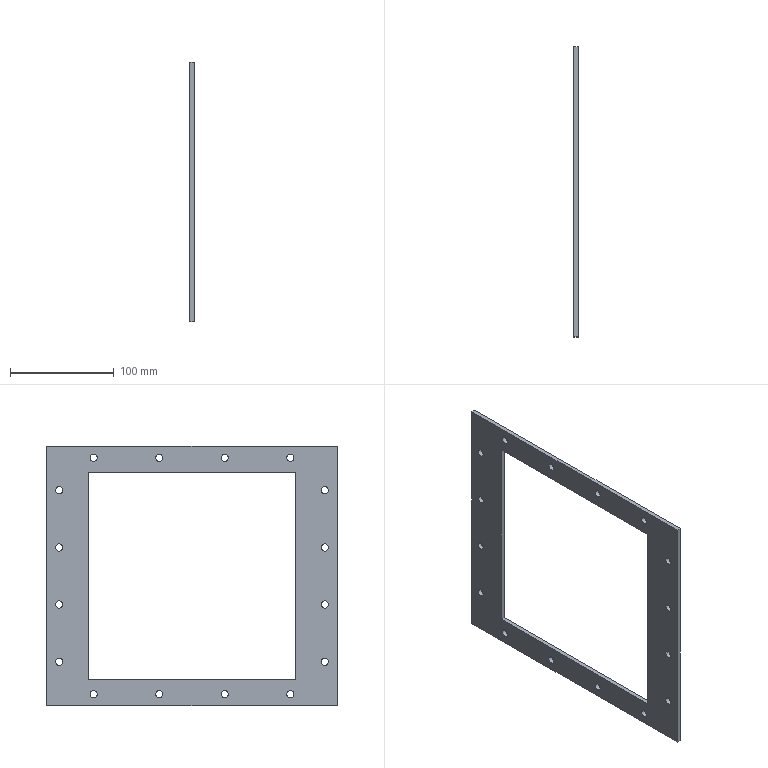Part | SolidWorks | features Boss 6, ICE 3, Revolution 3, CirPattern 2, Cut 2, Extrusion 1, MirrorPattern 1, RevCut 1, Shell 1 | 1 solid | 42 faces | box 4 x 280 x 250 mm | volume 117537 mm3 | cylinder 32 | plane 10 | commonest cylinder face diameters 7 x32
STEP:
#1=CARTESIAN_POINT('',(-187.,-320.5,-82.533));
#2=VERTEX_POINT('',#1);
#3=CARTESIAN_POINT('',(-187.,-327.5,-82.533));
#4=VERTEX_POINT('',#3);
#5=CARTESIAN_POINT('',(-187.,-324.,-82.533));
#6=DIRECTION('',(-1.,0.,0.));
#7=DIRECTION('',(0.,-1.,0.));
#8=AXIS2_PLACEMENT_3D('',#5,#6,#7);
#9=CIRCLE('',#8,3.5);
#10=EDGE_CURVE('',#2,#4,#9,.T.);
#11=ORIENTED_EDGE('',*,*,#10,.F.);
#12=CARTESIAN_POINT('',(-191.,-320.5,-82.533));
#13=VERTEX_POINT('',#12);
#14=CARTESIAN_POINT('',(-181.,-320.5,-82.533));
#15=DIRECTION('',(-1.,0.,0.));
#16=VECTOR('',#15,1000.);
#17=LINE('',#14,#16);
#18=EDGE_CURVE('',#2,#13,#17,.T.);
#19=ORIENTED_EDGE('',*,*,#18,.T.);
#20=CARTESIAN_POINT('',(-191.,-327.5,-82.533));
#21=VERTEX_POINT('',#20);
#22=CARTESIAN_POINT('',(-191.,-324.,-82.533));
#23=DIRECTION('',(-1.,0.,0.));
#24=DIRECTION('',(0.,1.,0.));
#25=AXIS2_PLACEMENT_3D('',#22,#23,#24);
#26=CIRCLE('',#25,3.5);
#27=EDGE_CURVE('',#13,#21,#26,.T.);
#28=ORIENTED_EDGE('',*,*,#27,.T.);
#29=CARTESIAN_POINT('',(-181.,-327.5,-82.533));
#30=DIRECTION('',(-1.,0.,0.));
#31=VECTOR('',#30,1000.);
#32=LINE('',#29,#31);
#33=EDGE_CURVE('',#4,#21,#32,.T.);
#34=ORIENTED_EDGE('',*,*,#33,.F.);
#35=EDGE_LOOP('',(#11,#19,#28,#34));
#36=FACE_OUTER_BOUND('',#35,.T.);
#37=CARTESIAN_POINT('',(-181.,-324.,-82.533));
#38=DIRECTION('',(-1.,0.,0.));
#39=DIRECTION('',(0.,-1.,0.));
#40=AXIS2_PLACEMENT_3D('',#37,#38,#39);
#41=CYLINDRICAL_SURFACE('',#40,3.5);
#42=ADVANCED_FACE('',(#36),#41,.F.);
#43=CARTESIAN_POINT('',(-187.,-320.5,-27.511));
#44=VERTEX_POINT('',#43);
#45=CARTESIAN_POINT('',(-187.,-327.5,-27.511));
#46=VERTEX_POINT('',#45);
#47=CARTESIAN_POINT('',(-187.,-324.,-27.511));
#48=DIRECTION('',(-1.,0.,0.));
#49=DIRECTION('',(0.,-1.,0.));
#50=AXIS2_PLACEMENT_3D('',#47,#48,#49);
#51=CIRCLE('',#50,3.5);
#52=EDGE_CURVE('',#44,#46,#51,.T.);
#53=ORIENTED_EDGE('',*,*,#52,.F.);
#54=CARTESIAN_POINT('',(-191.,-320.5,-27.511));
#55=VERTEX_POINT('',#54);
#56=CARTESIAN_POINT('',(-181.,-320.5,-27.511));
#57=DIRECTION('',(-1.,0.,0.));
#58=VECTOR('',#57,1000.);
#59=LINE('',#56,#58);
#60=EDGE_CURVE('',#44,#55,#59,.T.);
#61=ORIENTED_EDGE('',*,*,#60,.T.);
#62=CARTESIAN_POINT('',(-191.,-327.5,-27.511));
#63=VERTEX_POINT('',#62);
#64=CARTESIAN_POINT('',(-191.,-324.,-27.511));
#65=DIRECTION('',(-1.,0.,0.));
#66=DIRECTION('',(0.,1.,0.));
#67=AXIS2_PLACEMENT_3D('',#64,#65,#66);
#68=CIRCLE('',#67,3.5);
#69=EDGE_CURVE('',#55,#63,#68,.T.);
#70=ORIENTED_EDGE('',*,*,#69,.T.);
#71=CARTESIAN_POINT('',(-181.,-327.5,-27.511));
#72=DIRECTION('',(-1.,0.,0.));
#73=VECTOR('',#72,1000.);
#74=LINE('',#71,#73);
#75=EDGE_CURVE('',#46,#63,#74,.T.);
#76=ORIENTED_EDGE('',*,*,#75,.F.);
#77=EDGE_LOOP('',(#53,#61,#70,#76));
#78=FACE_OUTER_BOUND('',#77,.T.);
#79=CARTESIAN_POINT('',(-181.,-324.,-27.511));
#80=DIRECTION('',(-1.,0.,0.));
#81=DIRECTION('',(0.,-1.,0.));
#82=AXIS2_PLACEMENT_3D('',#79,#80,#81);
#83=CYLINDRICAL_SURFACE('',#82,3.5);
#84=ADVANCED_FACE('',(#78),#83,.F.);
#85=CARTESIAN_POINT('',(-187.,-320.5,27.511));
#86=VERTEX_POINT('',#85);
#87=CARTESIAN_POINT('',(-187.,-327.5,27.511));
#88=VERTEX_POINT('',#87);
#89=CARTESIAN_POINT('',(-187.,-324.,27.511));
#90=DIRECTION('',(-1.,0.,0.));
#91=DIRECTION('',(0.,-1.,0.));
#92=AXIS2_PLACEMENT_3D('',#89,#90,#91);
#93=CIRCLE('',#92,3.5);
#94=EDGE_CURVE('',#86,#88,#93,.T.);
#95=ORIENTED_EDGE('',*,*,#94,.F.);
#96=CARTESIAN_POINT('',(-191.,-320.5,27.511));
#97=VERTEX_POINT('',#96);
#98=CARTESIAN_POINT('',(-181.,-320.5,27.511));
#99=DIRECTION('',(-1.,0.,0.));
#100=VECTOR('',#99,1000.);
#101=LINE('',#98,#100);
#102=EDGE_CURVE('',#86,#97,#101,.T.);
#103=ORIENTED_EDGE('',*,*,#102,.T.);
#104=CARTESIAN_POINT('',(-191.,-327.5,27.511));
#105=VERTEX_POINT('',#104);
#106=CARTESIAN_POINT('',(-191.,-324.,27.511));
#107=DIRECTION('',(-1.,0.,0.));
#108=DIRECTION('',(0.,1.,0.));
#109=AXIS2_PLACEMENT_3D('',#106,#107,#108);
#110=CIRCLE('',#109,3.5);
#111=EDGE_CURVE('',#97,#105,#110,.T.);
#112=ORIENTED_EDGE('',*,*,#111,.T.);
#113=CARTESIAN_POINT('',(-181.,-327.5,27.511));
#114=DIRECTION('',(-1.,0.,0.));
#115=VECTOR('',#114,1000.);
#116=LINE('',#113,#115);
#117=EDGE_CURVE('',#88,#105,#116,.T.);
#118=ORIENTED_EDGE('',*,*,#117,.F.);
#119=EDGE_LOOP('',(#95,#103,#112,#118));
#120=FACE_OUTER_BOUND('',#119,.T.);
#121=CARTESIAN_POINT('',(-181.,-324.,27.511));
#122=DIRECTION('',(-1.,0.,0.));
#123=DIRECTION('',(0.,-1.,0.));
#124=AXIS2_PLACEMENT_3D('',#121,#122,#123);
#125=CYLINDRICAL_SURFACE('',#124,3.5);
#126=ADVANCED_FACE('',(#120),#125,.F.);
#127=CARTESIAN_POINT('',(-187.,-320.5,82.533));
#128=VERTEX_POINT('',#127);
#129=CARTESIAN_POINT('',(-187.,-327.5,82.533));
#130=VERTEX_POINT('',#129);
#131=CARTESIAN_POINT('',(-187.,-324.,82.533));
#132=DIRECTION('',(-1.,0.,0.));
#133=DIRECTION('',(0.,-1.,0.));
#134=AXIS2_PLACEMENT_3D('',#131,#132,#133);
#135=CIRCLE('',#134,3.5);
#136=EDGE_CURVE('',#128,#130,#135,.T.);
#137=ORIENTED_EDGE('',*,*,#136,.F.);
#138=CARTESIAN_POINT('',(-191.,-320.5,82.533));
#139=VERTEX_POINT('',#138);
#140=CARTESIAN_POINT('',(-181.,-320.5,82.533));
#141=DIRECTION('',(-1.,0.,0.));
#142=VECTOR('',#141,1000.);
#143=LINE('',#140,#142);
#144=EDGE_CURVE('',#128,#139,#143,.T.);
#145=ORIENTED_EDGE('',*,*,#144,.T.);
#146=CARTESIAN_POINT('',(-191.,-327.5,82.533));
#147=VERTEX_POINT('',#146);
#148=CARTESIAN_POINT('',(-191.,-324.,82.533));
#149=DIRECTION('',(-1.,0.,0.));
#150=DIRECTION('',(0.,1.,0.));
#151=AXIS2_PLACEMENT_3D('',#148,#149,#150);
#152=CIRCLE('',#151,3.5);
#153=EDGE_CURVE('',#139,#147,#152,.T.);
#154=ORIENTED_EDGE('',*,*,#153,.T.);
#155=CARTESIAN_POINT('',(-181.,-327.5,82.533));
#156=DIRECTION('',(-1.,0.,0.));
#157=VECTOR('',#156,1000.);
#158=LINE('',#155,#157);
#159=EDGE_CURVE('',#130,#147,#158,.T.);
#160=ORIENTED_EDGE('',*,*,#159,.F.);
#161=EDGE_LOOP('',(#137,#145,#154,#160));
#162=FACE_OUTER_BOUND('',#161,.T.);
#163=CARTESIAN_POINT('',(-181.,-324.,82.533));
#164=DIRECTION('',(-1.,0.,0.));
#165=DIRECTION('',(0.,-1.,0.));
#166=AXIS2_PLACEMENT_3D('',#163,#164,#165);
#167=CYLINDRICAL_SURFACE('',#166,3.5);
#168=ADVANCED_FACE('',(#162),#167,.F.);
#169=CARTESIAN_POINT('',(-187.,-97.719,114.));
#170=VERTEX_POINT('',#169);
#171=CARTESIAN_POINT('',(-187.,-104.719,114.));
#172=VERTEX_POINT('',#171);
#173=CARTESIAN_POINT('',(-187.,-101.219,114.));
#174=DIRECTION('',(-1.,0.,0.));
#175=DIRECTION('',(0.,-1.,0.));
#176=AXIS2_PLACEMENT_3D('',#173,#174,#175);
#177=CIRCLE('',#176,3.5);
#178=EDGE_CURVE('',#170,#172,#177,.T.);
#179=ORIENTED_EDGE('',*,*,#178,.F.);
#180=CARTESIAN_POINT('',(-191.,-97.719,114.));
#181=VERTEX_POINT('',#180);
#182=CARTESIAN_POINT('',(-181.,-97.719,114.));
#183=DIRECTION('',(-1.,0.,0.));
#184=VECTOR('',#183,1000.);
#185=LINE('',#182,#184);
#186=EDGE_CURVE('',#170,#181,#185,.T.);
#187=ORIENTED_EDGE('',*,*,#186,.T.);
#188=CARTESIAN_POINT('',(-191.,-104.719,114.));
#189=VERTEX_POINT('',#188);
#190=CARTESIAN_POINT('',(-191.,-101.219,114.));
#191=DIRECTION('',(-1.,0.,0.));
#192=DIRECTION('',(0.,1.,0.));
#193=AXIS2_PLACEMENT_3D('',#190,#191,#192);
#194=CIRCLE('',#193,3.5);
#195=EDGE_CURVE('',#181,#189,#194,.T.);
#196=ORIENTED_EDGE('',*,*,#195,.T.);
#197=CARTESIAN_POINT('',(-181.,-104.719,114.));
#198=DIRECTION('',(-1.,0.,0.));
#199=VECTOR('',#198,1000.);
#200=LINE('',#197,#199);
#201=EDGE_CURVE('',#172,#189,#200,.T.);
#202=ORIENTED_EDGE('',*,*,#201,.F.);
#203=EDGE_LOOP('',(#179,#187,#196,#202));
#204=FACE_OUTER_BOUND('',#203,.T.);
#205=CARTESIAN_POINT('',(-181.,-101.219,114.));
#206=DIRECTION('',(-1.,0.,0.));
#207=DIRECTION('',(0.,-1.,0.));
#208=AXIS2_PLACEMENT_3D('',#205,#206,#207);
#209=CYLINDRICAL_SURFACE('',#208,3.5);
#210=ADVANCED_FACE('',(#204),#209,.F.);
#211=CARTESIAN_POINT('',(-187.,-160.906,114.));
#212=VERTEX_POINT('',#211);
#213=CARTESIAN_POINT('',(-187.,-167.906,114.));
#214=VERTEX_POINT('',#213);
#215=CARTESIAN_POINT('',(-187.,-164.406,114.));
#216=DIRECTION('',(-1.,0.,0.));
#217=DIRECTION('',(0.,-1.,0.));
#218=AXIS2_PLACEMENT_3D('',#215,#216,#217);
#219=CIRCLE('',#218,3.5);
#220=EDGE_CURVE('',#212,#214,#219,.T.);
#221=ORIENTED_EDGE('',*,*,#220,.F.);
#222=CARTESIAN_POINT('',(-191.,-160.906,114.));
#223=VERTEX_POINT('',#222);
#224=CARTESIAN_POINT('',(-181.,-160.906,114.));
#225=DIRECTION('',(-1.,0.,0.));
#226=VECTOR('',#225,1000.);
#227=LINE('',#224,#226);
#228=EDGE_CURVE('',#212,#223,#227,.T.);
#229=ORIENTED_EDGE('',*,*,#228,.T.);
#230=CARTESIAN_POINT('',(-191.,-167.906,114.));
#231=VERTEX_POINT('',#230);
#232=CARTESIAN_POINT('',(-191.,-164.406,114.));
#233=DIRECTION('',(-1.,0.,0.));
#234=DIRECTION('',(0.,1.,0.));
#235=AXIS2_PLACEMENT_3D('',#232,#233,#234);
#236=CIRCLE('',#235,3.5);
#237=EDGE_CURVE('',#223,#231,#236,.T.);
#238=ORIENTED_EDGE('',*,*,#237,.T.);
#239=CARTESIAN_POINT('',(-181.,-167.906,114.));
#240=DIRECTION('',(-1.,0.,0.));
#241=VECTOR('',#240,1000.);
#242=LINE('',#239,#241);
#243=EDGE_CURVE('',#214,#231,#242,.T.);
#244=ORIENTED_EDGE('',*,*,#243,.F.);
#245=EDGE_LOOP('',(#221,#229,#238,#244));
#246=FACE_OUTER_BOUND('',#245,.T.);
#247=CARTESIAN_POINT('',(-181.,-164.406,114.));
#248=DIRECTION('',(-1.,0.,0.));
#249=DIRECTION('',(0.,-1.,0.));
#250=AXIS2_PLACEMENT_3D('',#247,#248,#249);
#251=CYLINDRICAL_SURFACE('',#250,3.5);
#252=ADVANCED_FACE('',(#246),#251,.F.);
#253=CARTESIAN_POINT('',(-187.,-224.094,114.));
#254=VERTEX_POINT('',#253);
#255=CARTESIAN_POINT('',(-187.,-231.094,114.));
#256=VERTEX_POINT('',#255);
#257=CARTESIAN_POINT('',(-187.,-227.594,114.));
#258=DIRECTION('',(-1.,0.,0.));
#259=DIRECTION('',(0.,-1.,0.));
#260=AXIS2_PLACEMENT_3D('',#257,#258,#259);
#261=CIRCLE('',#260,3.5);
#262=EDGE_CURVE('',#254,#256,#261,.T.);
#263=ORIENTED_EDGE('',*,*,#262,.F.);
#264=CARTESIAN_POINT('',(-191.,-224.094,114.));
#265=VERTEX_POINT('',#264);
#266=CARTESIAN_POINT('',(-181.,-224.094,114.));
#267=DIRECTION('',(-1.,0.,0.));
#268=VECTOR('',#267,1000.);
#269=LINE('',#266,#268);
#270=EDGE_CURVE('',#254,#265,#269,.T.);
#271=ORIENTED_EDGE('',*,*,#270,.T.);
#272=CARTESIAN_POINT('',(-191.,-231.094,114.));
#273=VERTEX_POINT('',#272);
#274=CARTESIAN_POINT('',(-191.,-227.594,114.));
#275=DIRECTION('',(-1.,0.,0.));
#276=DIRECTION('',(0.,1.,0.));
#277=AXIS2_PLACEMENT_3D('',#274,#275,#276);
#278=CIRCLE('',#277,3.5);
#279=EDGE_CURVE('',#265,#273,#278,.T.);
#280=ORIENTED_EDGE('',*,*,#279,.T.);
#281=CARTESIAN_POINT('',(-181.,-231.094,114.));
#282=DIRECTION('',(-1.,0.,0.));
#283=VECTOR('',#282,1000.);
#284=LINE('',#281,#283);
#285=EDGE_CURVE('',#256,#273,#284,.T.);
#286=ORIENTED_EDGE('',*,*,#285,.F.);
#287=EDGE_LOOP('',(#263,#271,#280,#286));
#288=FACE_OUTER_BOUND('',#287,.T.);
#289=CARTESIAN_POINT('',(-181.,-227.594,114.));
#290=DIRECTION('',(-1.,0.,0.));
#291=DIRECTION('',(0.,-1.,0.));
#292=AXIS2_PLACEMENT_3D('',#289,#290,#291);
#293=CYLINDRICAL_SURFACE('',#292,3.5);
#294=ADVANCED_FACE('',(#288),#293,.F.);
#295=CARTESIAN_POINT('',(-187.,-287.281,-114.));
#296=VERTEX_POINT('',#295);
#297=CARTESIAN_POINT('',(-187.,-294.281,-114.));
#298=VERTEX_POINT('',#297);
#299=CARTESIAN_POINT('',(-187.,-290.781,-114.));
#300=DIRECTION('',(-1.,0.,0.));
#301=DIRECTION('',(0.,-1.,0.));
#302=AXIS2_PLACEMENT_3D('',#299,#300,#301);
#303=CIRCLE('',#302,3.5);
#304=EDGE_CURVE('',#296,#298,#303,.T.);
#305=ORIENTED_EDGE('',*,*,#304,.F.);
#306=CARTESIAN_POINT('',(-191.,-287.281,-114.));
#307=VERTEX_POINT('',#306);
#308=CARTESIAN_POINT('',(-181.,-287.281,-114.));
#309=DIRECTION('',(-1.,0.,0.));
#310=VECTOR('',#309,1000.);
#311=LINE('',#308,#310);
#312=EDGE_CURVE('',#296,#307,#311,.T.);
#313=ORIENTED_EDGE('',*,*,#312,.T.);
#314=CARTESIAN_POINT('',(-191.,-294.281,-114.));
#315=VERTEX_POINT('',#314);
#316=CARTESIAN_POINT('',(-191.,-290.781,-114.));
#317=DIRECTION('',(-1.,0.,0.));
#318=DIRECTION('',(0.,-1.,0.));
#319=AXIS2_PLACEMENT_3D('',#316,#317,#318);
#320=CIRCLE('',#319,3.5);
#321=EDGE_CURVE('',#307,#315,#320,.T.);
#322=ORIENTED_EDGE('',*,*,#321,.T.);
#323=CARTESIAN_POINT('',(-181.,-294.281,-114.));
#324=DIRECTION('',(-1.,0.,0.));
#325=VECTOR('',#324,1000.);
#326=LINE('',#323,#325);
#327=EDGE_CURVE('',#298,#315,#326,.T.);
#328=ORIENTED_EDGE('',*,*,#327,.F.);
#329=EDGE_LOOP('',(#305,#313,#322,#328));
#330=FACE_OUTER_BOUND('',#329,.T.);
#331=CARTESIAN_POINT('',(-181.,-290.781,-114.));
#332=DIRECTION('',(-1.,0.,0.));
#333=DIRECTION('',(0.,-1.,0.));
#334=AXIS2_PLACEMENT_3D('',#331,#332,#333);
#335=CYLINDRICAL_SURFACE('',#334,3.5);
#336=ADVANCED_FACE('',(#330),#335,.F.);
#337=CARTESIAN_POINT('',(-187.,-224.094,-114.));
#338=VERTEX_POINT('',#337);
#339=CARTESIAN_POINT('',(-187.,-231.094,-114.));
#340=VERTEX_POINT('',#339);
#341=CARTESIAN_POINT('',(-187.,-227.594,-114.));
#342=DIRECTION('',(-1.,0.,0.));
#343=DIRECTION('',(0.,-1.,0.));
#344=AXIS2_PLACEMENT_3D('',#341,#342,#343);
#345=CIRCLE('',#344,3.5);
#346=EDGE_CURVE('',#338,#340,#345,.T.);
#347=ORIENTED_EDGE('',*,*,#346,.F.);
#348=CARTESIAN_POINT('',(-191.,-224.094,-114.));
#349=VERTEX_POINT('',#348);
#350=CARTESIAN_POINT('',(-181.,-224.094,-114.));
#351=DIRECTION('',(-1.,0.,0.));
#352=VECTOR('',#351,1000.);
#353=LINE('',#350,#352);
#354=EDGE_CURVE('',#338,#349,#353,.T.);
#355=ORIENTED_EDGE('',*,*,#354,.T.);
#356=CARTESIAN_POINT('',(-191.,-231.094,-114.));
#357=VERTEX_POINT('',#356);
#358=CARTESIAN_POINT('',(-191.,-227.594,-114.));
#359=DIRECTION('',(-1.,0.,0.));
#360=DIRECTION('',(0.,-1.,0.));
#361=AXIS2_PLACEMENT_3D('',#358,#359,#360);
#362=CIRCLE('',#361,3.5);
#363=EDGE_CURVE('',#349,#357,#362,.T.);
#364=ORIENTED_EDGE('',*,*,#363,.T.);
#365=CARTESIAN_POINT('',(-181.,-231.094,-114.));
#366=DIRECTION('',(-1.,0.,0.));
#367=VECTOR('',#366,1000.);
#368=LINE('',#365,#367);
#369=EDGE_CURVE('',#340,#357,#368,.T.);
#370=ORIENTED_EDGE('',*,*,#369,.F.);
#371=EDGE_LOOP('',(#347,#355,#364,#370));
#372=FACE_OUTER_BOUND('',#371,.T.);
#373=CARTESIAN_POINT('',(-181.,-227.594,-114.));
#374=DIRECTION('',(-1.,0.,0.));
#375=DIRECTION('',(0.,-1.,0.));
#376=AXIS2_PLACEMENT_3D('',#373,#374,#375);
#377=CYLINDRICAL_SURFACE('',#376,3.5);
#378=ADVANCED_FACE('',(#372),#377,.F.);
#379=CARTESIAN_POINT('',(-187.,-160.906,-114.));
#380=VERTEX_POINT('',#379);
#381=CARTESIAN_POINT('',(-187.,-167.906,-114.));
#382=VERTEX_POINT('',#381);
#383=CARTESIAN_POINT('',(-187.,-164.406,-114.));
#384=DIRECTION('',(-1.,0.,0.));
#385=DIRECTION('',(0.,-1.,0.));
#386=AXIS2_PLACEMENT_3D('',#383,#384,#385);
#387=CIRCLE('',#386,3.5);
#388=EDGE_CURVE('',#380,#382,#387,.T.);
#389=ORIENTED_EDGE('',*,*,#388,.F.);
#390=CARTESIAN_POINT('',(-191.,-160.906,-114.));
#391=VERTEX_POINT('',#390);
#392=CARTESIAN_POINT('',(-181.,-160.906,-114.));
#393=DIRECTION('',(-1.,0.,0.));
#394=VECTOR('',#393,1000.);
#395=LINE('',#392,#394);
#396=EDGE_CURVE('',#380,#391,#395,.T.);
#397=ORIENTED_EDGE('',*,*,#396,.T.);
#398=CARTESIAN_POINT('',(-191.,-167.906,-114.));
#399=VERTEX_POINT('',#398);
#400=CARTESIAN_POINT('',(-191.,-164.406,-114.));
#401=DIRECTION('',(-1.,0.,0.));
#402=DIRECTION('',(0.,-1.,0.));
#403=AXIS2_PLACEMENT_3D('',#400,#401,#402);
#404=CIRCLE('',#403,3.5);
#405=EDGE_CURVE('',#391,#399,#404,.T.);
#406=ORIENTED_EDGE('',*,*,#405,.T.);
#407=CARTESIAN_POINT('',(-181.,-167.906,-114.));
#408=DIRECTION('',(-1.,0.,0.));
#409=VECTOR('',#408,1000.);
#410=LINE('',#407,#409);
#411=EDGE_CURVE('',#382,#399,#410,.T.);
#412=ORIENTED_EDGE('',*,*,#411,.F.);
#413=EDGE_LOOP('',(#389,#397,#406,#412));
#414=FACE_OUTER_BOUND('',#413,.T.);
#415=CARTESIAN_POINT('',(-181.,-164.406,-114.));
#416=DIRECTION('',(-1.,0.,0.));
#417=DIRECTION('',(0.,-1.,0.));
#418=AXIS2_PLACEMENT_3D('',#415,#416,#417);
#419=CYLINDRICAL_SURFACE('',#418,3.5);
#420=ADVANCED_FACE('',(#414),#419,.F.);
#421=CARTESIAN_POINT('',(-187.,-287.281,114.));
#422=VERTEX_POINT('',#421);
#423=CARTESIAN_POINT('',(-187.,-294.281,114.));
#424=VERTEX_POINT('',#423);
#425=CARTESIAN_POINT('',(-187.,-290.781,114.));
#426=DIRECTION('',(-1.,0.,0.));
#427=DIRECTION('',(0.,-1.,0.));
#428=AXIS2_PLACEMENT_3D('',#425,#426,#427);
#429=CIRCLE('',#428,3.5);
#430=EDGE_CURVE('',#422,#424,#429,.T.);
#431=ORIENTED_EDGE('',*,*,#430,.F.);
#432=CARTESIAN_POINT('',(-191.,-287.281,114.));
#433=VERTEX_POINT('',#432);
#434=CARTESIAN_POINT('',(-181.,-287.281,114.));
#435=DIRECTION('',(-1.,0.,0.));
#436=VECTOR('',#435,1000.);
#437=LINE('',#434,#436);
#438=EDGE_CURVE('',#422,#433,#437,.T.);
#439=ORIENTED_EDGE('',*,*,#438,.T.);
#440=CARTESIAN_POINT('',(-191.,-294.281,114.));
#441=VERTEX_POINT('',#440);
#442=CARTESIAN_POINT('',(-191.,-290.781,114.));
#443=DIRECTION('',(-1.,0.,0.));
#444=DIRECTION('',(0.,1.,0.));
#445=AXIS2_PLACEMENT_3D('',#442,#443,#444);
#446=CIRCLE('',#445,3.5);
#447=EDGE_CURVE('',#433,#441,#446,.T.);
#448=ORIENTED_EDGE('',*,*,#447,.T.);
#449=CARTESIAN_POINT('',(-181.,-294.281,114.));
#450=DIRECTION('',(-1.,0.,0.));
#451=VECTOR('',#450,1000.);
#452=LINE('',#449,#451);
#453=EDGE_CURVE('',#424,#441,#452,.T.);
#454=ORIENTED_EDGE('',*,*,#453,.F.);
#455=EDGE_LOOP('',(#431,#439,#448,#454));
#456=FACE_OUTER_BOUND('',#455,.T.);
#457=CARTESIAN_POINT('',(-181.,-290.781,114.));
#458=DIRECTION('',(-1.,0.,0.));
#459=DIRECTION('',(0.,-1.,0.));
#460=AXIS2_PLACEMENT_3D('',#457,#458,#459);
#461=CYLINDRICAL_SURFACE('',#460,3.5);
#462=ADVANCED_FACE('',(#456),#461,.F.);
#463=CARTESIAN_POINT('',(-187.,-97.719,-114.));
#464=VERTEX_POINT('',#463);
#465=CARTESIAN_POINT('',(-187.,-104.719,-114.));
#466=VERTEX_POINT('',#465);
#467=CARTESIAN_POINT('',(-187.,-101.219,-114.));
#468=DIRECTION('',(-1.,0.,0.));
#469=DIRECTION('',(0.,-1.,0.));
#470=AXIS2_PLACEMENT_3D('',#467,#468,#469);
#471=CIRCLE('',#470,3.5);
#472=EDGE_CURVE('',#464,#466,#471,.T.);
#473=ORIENTED_EDGE('',*,*,#472,.F.);
#474=CARTESIAN_POINT('',(-191.,-97.719,-114.));
#475=VERTEX_POINT('',#474);
#476=CARTESIAN_POINT('',(-181.,-97.719,-114.));
#477=DIRECTION('',(-1.,0.,0.));
#478=VECTOR('',#477,1000.);
#479=LINE('',#476,#478);
#480=EDGE_CURVE('',#464,#475,#479,.T.);
#481=ORIENTED_EDGE('',*,*,#480,.T.);
#482=CARTESIAN_POINT('',(-191.,-104.719,-114.));
#483=VERTEX_POINT('',#482);
#484=CARTESIAN_POINT('',(-191.,-101.219,-114.));
#485=DIRECTION('',(-1.,0.,0.));
#486=DIRECTION('',(0.,-1.,0.));
#487=AXIS2_PLACEMENT_3D('',#484,#485,#486);
#488=CIRCLE('',#487,3.5);
#489=EDGE_CURVE('',#475,#483,#488,.T.);
#490=ORIENTED_EDGE('',*,*,#489,.T.);
#491=CARTESIAN_POINT('',(-181.,-104.719,-114.));
#492=DIRECTION('',(-1.,0.,0.));
#493=VECTOR('',#492,1000.);
#494=LINE('',#491,#493);
#495=EDGE_CURVE('',#466,#483,#494,.T.);
#496=ORIENTED_EDGE('',*,*,#495,.F.);
#497=EDGE_LOOP('',(#473,#481,#490,#496));
#498=FACE_OUTER_BOUND('',#497,.T.);
#499=CARTESIAN_POINT('',(-181.,-101.219,-114.));
#500=DIRECTION('',(-1.,0.,0.));
#501=DIRECTION('',(0.,-1.,0.));
#502=AXIS2_PLACEMENT_3D('',#499,#500,#501);
#503=CYLINDRICAL_SURFACE('',#502,3.5);
#504=ADVANCED_FACE('',(#498),#503,.F.);
#505=CARTESIAN_POINT('',(-187.,-64.5,82.533));
#506=VERTEX_POINT('',#505);
#507=CARTESIAN_POINT('',(-187.,-71.5,82.533));
#508=VERTEX_POINT('',#507);
#509=CARTESIAN_POINT('',(-187.,-68.,82.533));
#510=DIRECTION('',(-1.,0.,0.));
#511=DIRECTION('',(0.,1.,0.));
#512=AXIS2_PLACEMENT_3D('',#509,#510,#511);
#513=CIRCLE('',#512,3.5);
#514=EDGE_CURVE('',#506,#508,#513,.T.);
#515=ORIENTED_EDGE('',*,*,#514,.F.);
#516=CARTESIAN_POINT('',(-191.,-64.5,82.533));
#517=VERTEX_POINT('',#516);
#518=CARTESIAN_POINT('',(-181.,-64.5,82.533));
#519=DIRECTION('',(-1.,0.,0.));
#520=VECTOR('',#519,1000.);
#521=LINE('',#518,#520);
#522=EDGE_CURVE('',#506,#517,#521,.T.);
#523=ORIENTED_EDGE('',*,*,#522,.T.);
#524=CARTESIAN_POINT('',(-191.,-71.5,82.533));
#525=VERTEX_POINT('',#524);
#526=CARTESIAN_POINT('',(-191.,-68.,82.533));
#527=DIRECTION('',(-1.,0.,0.));
#528=DIRECTION('',(0.,-1.,0.));
#529=AXIS2_PLACEMENT_3D('',#526,#527,#528);
#530=CIRCLE('',#529,3.5);
#531=EDGE_CURVE('',#517,#525,#530,.T.);
#532=ORIENTED_EDGE('',*,*,#531,.T.);
#533=CARTESIAN_POINT('',(-181.,-71.5,82.533));
#534=DIRECTION('',(-1.,0.,0.));
#535=VECTOR('',#534,1000.);
#536=LINE('',#533,#535);
#537=EDGE_CURVE('',#508,#525,#536,.T.);
#538=ORIENTED_EDGE('',*,*,#537,.F.);
#539=EDGE_LOOP('',(#515,#523,#532,#538));
#540=FACE_OUTER_BOUND('',#539,.T.);
#541=CARTESIAN_POINT('',(-181.,-68.,82.533));
#542=DIRECTION('',(-1.,0.,0.));
#543=DIRECTION('',(0.,-1.,0.));
#544=AXIS2_PLACEMENT_3D('',#541,#542,#543);
#545=CYLINDRICAL_SURFACE('',#544,3.5);
#546=ADVANCED_FACE('',(#540),#545,.F.);
#547=CARTESIAN_POINT('',(-187.,-64.5,27.511));
#548=VERTEX_POINT('',#547);
#549=CARTESIAN_POINT('',(-187.,-71.5,27.511));
#550=VERTEX_POINT('',#549);
#551=CARTESIAN_POINT('',(-187.,-68.,27.511));
#552=DIRECTION('',(-1.,0.,0.));
#553=DIRECTION('',(0.,1.,0.));
#554=AXIS2_PLACEMENT_3D('',#551,#552,#553);
#555=CIRCLE('',#554,3.5);
#556=EDGE_CURVE('',#548,#550,#555,.T.);
#557=ORIENTED_EDGE('',*,*,#556,.F.);
#558=CARTESIAN_POINT('',(-191.,-64.5,27.511));
#559=VERTEX_POINT('',#558);
#560=CARTESIAN_POINT('',(-181.,-64.5,27.511));
#561=DIRECTION('',(-1.,0.,0.));
#562=VECTOR('',#561,1000.);
#563=LINE('',#560,#562);
#564=EDGE_CURVE('',#548,#559,#563,.T.);
#565=ORIENTED_EDGE('',*,*,#564,.T.);
#566=CARTESIAN_POINT('',(-191.,-71.5,27.511));
#567=VERTEX_POINT('',#566);
#568=CARTESIAN_POINT('',(-191.,-68.,27.511));
#569=DIRECTION('',(-1.,0.,0.));
#570=DIRECTION('',(0.,-1.,0.));
#571=AXIS2_PLACEMENT_3D('',#568,#569,#570);
#572=CIRCLE('',#571,3.5);
#573=EDGE_CURVE('',#559,#567,#572,.T.);
#574=ORIENTED_EDGE('',*,*,#573,.T.);
#575=CARTESIAN_POINT('',(-181.,-71.5,27.511));
#576=DIRECTION('',(-1.,0.,0.));
#577=VECTOR('',#576,1000.);
#578=LINE('',#575,#577);
#579=EDGE_CURVE('',#550,#567,#578,.T.);
#580=ORIENTED_EDGE('',*,*,#579,.F.);
#581=EDGE_LOOP('',(#557,#565,#574,#580));
#582=FACE_OUTER_BOUND('',#581,.T.);
#583=CARTESIAN_POINT('',(-181.,-68.,27.511));
#584=DIRECTION('',(-1.,0.,0.));
#585=DIRECTION('',(0.,-1.,0.));
#586=AXIS2_PLACEMENT_3D('',#583,#584,#585);
#587=CYLINDRICAL_SURFACE('',#586,3.5);
#588=ADVANCED_FACE('',(#582),#587,.F.);
#589=CARTESIAN_POINT('',(-187.,-64.5,-27.511));
#590=VERTEX_POINT('',#589);
#591=CARTESIAN_POINT('',(-187.,-71.5,-27.511));
#592=VERTEX_POINT('',#591);
#593=CARTESIAN_POINT('',(-187.,-68.,-27.511));
#594=DIRECTION('',(-1.,0.,0.));
#595=DIRECTION('',(0.,1.,0.));
#596=AXIS2_PLACEMENT_3D('',#593,#594,#595);
#597=CIRCLE('',#596,3.5);
#598=EDGE_CURVE('',#590,#592,#597,.T.);
#599=ORIENTED_EDGE('',*,*,#598,.F.);
#600=CARTESIAN_POINT('',(-191.,-64.5,-27.511));
#601=VERTEX_POINT('',#600);
#602=CARTESIAN_POINT('',(-181.,-64.5,-27.511));
#603=DIRECTION('',(-1.,0.,0.));
#604=VECTOR('',#603,1000.);
#605=LINE('',#602,#604);
#606=EDGE_CURVE('',#590,#601,#605,.T.);
#607=ORIENTED_EDGE('',*,*,#606,.T.);
#608=CARTESIAN_POINT('',(-191.,-71.5,-27.511));
#609=VERTEX_POINT('',#608);
#610=CARTESIAN_POINT('',(-191.,-68.,-27.511));
#611=DIRECTION('',(-1.,0.,0.));
#612=DIRECTION('',(0.,-1.,0.));
#613=AXIS2_PLACEMENT_3D('',#610,#611,#612);
#614=CIRCLE('',#613,3.5);
#615=EDGE_CURVE('',#601,#609,#614,.T.);
#616=ORIENTED_EDGE('',*,*,#615,.T.);
#617=CARTESIAN_POINT('',(-181.,-71.5,-27.511));
#618=DIRECTION('',(-1.,0.,0.));
#619=VECTOR('',#618,1000.);
#620=LINE('',#617,#619);
#621=EDGE_CURVE('',#592,#609,#620,.T.);
#622=ORIENTED_EDGE('',*,*,#621,.F.);
#623=EDGE_LOOP('',(#599,#607,#616,#622));
#624=FACE_OUTER_BOUND('',#623,.T.);
#625=CARTESIAN_POINT('',(-181.,-68.,-27.511));
#626=DIRECTION('',(-1.,0.,0.));
#627=DIRECTION('',(0.,-1.,0.));
#628=AXIS2_PLACEMENT_3D('',#625,#626,#627);
#629=CYLINDRICAL_SURFACE('',#628,3.5);
#630=ADVANCED_FACE('',(#624),#629,.F.);
#631=CARTESIAN_POINT('',(-187.,-64.5,-82.533));
#632=VERTEX_POINT('',#631);
#633=CARTESIAN_POINT('',(-187.,-71.5,-82.533));
#634=VERTEX_POINT('',#633);
#635=CARTESIAN_POINT('',(-187.,-68.,-82.533));
#636=DIRECTION('',(-1.,0.,0.));
#637=DIRECTION('',(0.,1.,0.));
#638=AXIS2_PLACEMENT_3D('',#635,#636,#637);
#639=CIRCLE('',#638,3.5);
#640=EDGE_CURVE('',#632,#634,#639,.T.);
#641=ORIENTED_EDGE('',*,*,#640,.F.);
#642=CARTESIAN_POINT('',(-191.,-64.5,-82.533));
#643=VERTEX_POINT('',#642);
#644=CARTESIAN_POINT('',(-181.,-64.5,-82.533));
#645=DIRECTION('',(-1.,0.,0.));
#646=VECTOR('',#645,1000.);
#647=LINE('',#644,#646);
#648=EDGE_CURVE('',#632,#643,#647,.T.);
#649=ORIENTED_EDGE('',*,*,#648,.T.);
#650=CARTESIAN_POINT('',(-191.,-71.5,-82.533));
#651=VERTEX_POINT('',#650);
#652=CARTESIAN_POINT('',(-191.,-68.,-82.533));
#653=DIRECTION('',(-1.,0.,0.));
#654=DIRECTION('',(0.,-1.,0.));
#655=AXIS2_PLACEMENT_3D('',#652,#653,#654);
#656=CIRCLE('',#655,3.5);
#657=EDGE_CURVE('',#643,#651,#656,.T.);
#658=ORIENTED_EDGE('',*,*,#657,.T.);
#659=CARTESIAN_POINT('',(-181.,-71.5,-82.533));
#660=DIRECTION('',(-1.,0.,0.));
#661=VECTOR('',#660,1000.);
#662=LINE('',#659,#661);
#663=EDGE_CURVE('',#634,#651,#662,.T.);
#664=ORIENTED_EDGE('',*,*,#663,.F.);
#665=EDGE_LOOP('',(#641,#649,#658,#664));
#666=FACE_OUTER_BOUND('',#665,.T.);
#667=CARTESIAN_POINT('',(-181.,-68.,-82.533));
#668=DIRECTION('',(-1.,0.,0.));
#669=DIRECTION('',(0.,-1.,0.));
#670=AXIS2_PLACEMENT_3D('',#667,#668,#669);
#671=CYLINDRICAL_SURFACE('',#670,3.5);
#672=ADVANCED_FACE('',(#666),#671,.F.);
#673=CARTESIAN_POINT('',(-187.,-96.,-100.));
#674=VERTEX_POINT('',#673);
#675=CARTESIAN_POINT('',(-187.,-96.,100.));
#676=VERTEX_POINT('',#675);
#677=CARTESIAN_POINT('',(-187.,-96.,-98.));
#678=DIRECTION('',(0.,0.,1.));
#679=VECTOR('',#678,1000.);
#680=LINE('',#677,#679);
#681=EDGE_CURVE('',#674,#676,#680,.T.);
#682=ORIENTED_EDGE('',*,*,#681,.F.);
#683=CARTESIAN_POINT('',(-187.,-296.,-100.));
#684=VERTEX_POINT('',#683);
#685=CARTESIAN_POINT('',(-187.,-336.,-100.));
#686=DIRECTION('',(0.,-1.,0.));
#687=VECTOR('',#686,1000.);
#688=LINE('',#685,#687);
#689=EDGE_CURVE('',#674,#684,#688,.T.);
#690=ORIENTED_EDGE('',*,*,#689,.T.);
#691=CARTESIAN_POINT('',(-187.,-296.,100.));
#692=VERTEX_POINT('',#691);
#693=CARTESIAN_POINT('',(-187.,-296.,-98.));
#694=DIRECTION('',(0.,0.,1.));
#695=VECTOR('',#694,1000.);
#696=LINE('',#693,#695);
#697=EDGE_CURVE('',#684,#692,#696,.T.);
#698=ORIENTED_EDGE('',*,*,#697,.T.);
#699=CARTESIAN_POINT('',(-187.,-336.,100.));
#700=DIRECTION('',(0.,1.,0.));
#701=VECTOR('',#700,1000.);
#702=LINE('',#699,#701);
#703=EDGE_CURVE('',#692,#676,#702,.T.);
#704=ORIENTED_EDGE('',*,*,#703,.T.);
#705=EDGE_LOOP('',(#682,#690,#698,#704));
#706=FACE_BOUND('',#705,.T.);
#707=CARTESIAN_POINT('',(-187.,-324.,-82.533));
#708=DIRECTION('',(-1.,0.,0.));
#709=DIRECTION('',(0.,-1.,0.));
#710=AXIS2_PLACEMENT_3D('',#707,#708,#709);
#711=CIRCLE('',#710,3.5);
#712=EDGE_CURVE('',#4,#2,#711,.T.);
#713=ORIENTED_EDGE('',*,*,#712,.T.);
#714=ORIENTED_EDGE('',*,*,#10,.T.);
#715=EDGE_LOOP('',(#713,#714));
#716=FACE_BOUND('',#715,.T.);
#717=CARTESIAN_POINT('',(-187.,-324.,-27.511));
#718=DIRECTION('',(-1.,0.,0.));
#719=DIRECTION('',(0.,-1.,0.));
#720=AXIS2_PLACEMENT_3D('',#717,#718,#719);
#721=CIRCLE('',#720,3.5);
#722=EDGE_CURVE('',#46,#44,#721,.T.);
#723=ORIENTED_EDGE('',*,*,#722,.T.);
#724=ORIENTED_EDGE('',*,*,#52,.T.);
#725=EDGE_LOOP('',(#723,#724));
#726=FACE_BOUND('',#725,.T.);
#727=CARTESIAN_POINT('',(-187.,-324.,27.511));
#728=DIRECTION('',(-1.,0.,0.));
#729=DIRECTION('',(0.,-1.,0.));
#730=AXIS2_PLACEMENT_3D('',#727,#728,#729);
#731=CIRCLE('',#730,3.5);
#732=EDGE_CURVE('',#88,#86,#731,.T.);
#733=ORIENTED_EDGE('',*,*,#732,.T.);
#734=ORIENTED_EDGE('',*,*,#94,.T.);
#735=EDGE_LOOP('',(#733,#734));
#736=FACE_BOUND('',#735,.T.);
#737=CARTESIAN_POINT('',(-187.,-324.,82.533));
#738=DIRECTION('',(-1.,0.,0.));
#739=DIRECTION('',(0.,-1.,0.));
#740=AXIS2_PLACEMENT_3D('',#737,#738,#739);
#741=CIRCLE('',#740,3.5);
#742=EDGE_CURVE('',#130,#128,#741,.T.);
#743=ORIENTED_EDGE('',*,*,#742,.T.);
#744=ORIENTED_EDGE('',*,*,#136,.T.);
#745=EDGE_LOOP('',(#743,#744));
#746=FACE_BOUND('',#745,.T.);
#747=CARTESIAN_POINT('',(-187.,-101.219,114.));
#748=DIRECTION('',(-1.,0.,0.));
#749=DIRECTION('',(0.,-1.,0.));
#750=AXIS2_PLACEMENT_3D('',#747,#748,#749);
#751=CIRCLE('',#750,3.5);
#752=EDGE_CURVE('',#172,#170,#751,.T.);
#753=ORIENTED_EDGE('',*,*,#752,.T.);
#754=ORIENTED_EDGE('',*,*,#178,.T.);
#755=EDGE_LOOP('',(#753,#754));
#756=FACE_BOUND('',#755,.T.);
#757=CARTESIAN_POINT('',(-187.,-164.406,114.));
#758=DIRECTION('',(-1.,0.,0.));
#759=DIRECTION('',(0.,-1.,0.));
#760=AXIS2_PLACEMENT_3D('',#757,#758,#759);
#761=CIRCLE('',#760,3.5);
#762=EDGE_CURVE('',#214,#212,#761,.T.);
#763=ORIENTED_EDGE('',*,*,#762,.T.);
#764=ORIENTED_EDGE('',*,*,#220,.T.);
#765=EDGE_LOOP('',(#763,#764));
#766=FACE_BOUND('',#765,.T.);
#767=CARTESIAN_POINT('',(-187.,-227.594,114.));
#768=DIRECTION('',(-1.,0.,0.));
#769=DIRECTION('',(0.,-1.,0.));
#770=AXIS2_PLACEMENT_3D('',#767,#768,#769);
#771=CIRCLE('',#770,3.5);
#772=EDGE_CURVE('',#256,#254,#771,.T.);
#773=ORIENTED_EDGE('',*,*,#772,.T.);
#774=ORIENTED_EDGE('',*,*,#262,.T.);
#775=EDGE_LOOP('',(#773,#774));
#776=FACE_BOUND('',#775,.T.);
#777=CARTESIAN_POINT('',(-187.,-290.781,-114.));
#778=DIRECTION('',(-1.,0.,0.));
#779=DIRECTION('',(0.,-1.,0.));
#780=AXIS2_PLACEMENT_3D('',#777,#778,#779);
#781=CIRCLE('',#780,3.5);
#782=EDGE_CURVE('',#298,#296,#781,.T.);
#783=ORIENTED_EDGE('',*,*,#782,.T.);
#784=ORIENTED_EDGE('',*,*,#304,.T.);
#785=EDGE_LOOP('',(#783,#784));
#786=FACE_BOUND('',#785,.T.);
#787=CARTESIAN_POINT('',(-187.,-227.594,-114.));
#788=DIRECTION('',(-1.,0.,0.));
#789=DIRECTION('',(0.,-1.,0.));
#790=AXIS2_PLACEMENT_3D('',#787,#788,#789);
#791=CIRCLE('',#790,3.5);
#792=EDGE_CURVE('',#340,#338,#791,.T.);
#793=ORIENTED_EDGE('',*,*,#792,.T.);
#794=ORIENTED_EDGE('',*,*,#346,.T.);
#795=EDGE_LOOP('',(#793,#794));
#796=FACE_BOUND('',#795,.T.);
#797=CARTESIAN_POINT('',(-187.,-164.406,-114.));
#798=DIRECTION('',(-1.,0.,0.));
#799=DIRECTION('',(0.,-1.,0.));
#800=AXIS2_PLACEMENT_3D('',#797,#798,#799);
#801=CIRCLE('',#800,3.5);
#802=EDGE_CURVE('',#382,#380,#801,.T.);
#803=ORIENTED_EDGE('',*,*,#802,.T.);
#804=ORIENTED_EDGE('',*,*,#388,.T.);
#805=EDGE_LOOP('',(#803,#804));
#806=FACE_BOUND('',#805,.T.);
#807=CARTESIAN_POINT('',(-187.,-290.781,114.));
#808=DIRECTION('',(-1.,0.,0.));
#809=DIRECTION('',(0.,-1.,0.));
#810=AXIS2_PLACEMENT_3D('',#807,#808,#809);
#811=CIRCLE('',#810,3.5);
#812=EDGE_CURVE('',#424,#422,#811,.T.);
#813=ORIENTED_EDGE('',*,*,#812,.T.);
#814=ORIENTED_EDGE('',*,*,#430,.T.);
#815=EDGE_LOOP('',(#813,#814));
#816=FACE_BOUND('',#815,.T.);
#817=CARTESIAN_POINT('',(-187.,-101.219,-114.));
#818=DIRECTION('',(-1.,0.,0.));
#819=DIRECTION('',(0.,-1.,0.));
#820=AXIS2_PLACEMENT_3D('',#817,#818,#819);
#821=CIRCLE('',#820,3.5);
#822=EDGE_CURVE('',#466,#464,#821,.T.);
#823=ORIENTED_EDGE('',*,*,#822,.T.);
#824=ORIENTED_EDGE('',*,*,#472,.T.);
#825=EDGE_LOOP('',(#823,#824));
#826=FACE_BOUND('',#825,.T.);
#827=CARTESIAN_POINT('',(-187.,-68.,-82.533));
#828=DIRECTION('',(-1.,0.,0.));
#829=DIRECTION('',(0.,1.,0.));
#830=AXIS2_PLACEMENT_3D('',#827,#828,#829);
#831=CIRCLE('',#830,3.5);
#832=EDGE_CURVE('',#634,#632,#831,.T.);
#833=ORIENTED_EDGE('',*,*,#832,.T.);
#834=ORIENTED_EDGE('',*,*,#640,.T.);
#835=EDGE_LOOP('',(#833,#834));
#836=FACE_BOUND('',#835,.T.);
#837=CARTESIAN_POINT('',(-187.,-68.,-27.511));
#838=DIRECTION('',(-1.,0.,0.));
#839=DIRECTION('',(0.,1.,0.));
#840=AXIS2_PLACEMENT_3D('',#837,#838,#839);
#841=CIRCLE('',#840,3.5);
#842=EDGE_CURVE('',#592,#590,#841,.T.);
#843=ORIENTED_EDGE('',*,*,#842,.T.);
#844=ORIENTED_EDGE('',*,*,#598,.T.);
#845=EDGE_LOOP('',(#843,#844));
#846=FACE_BOUND('',#845,.T.);
#847=CARTESIAN_POINT('',(-187.,-68.,82.533));
#848=DIRECTION('',(-1.,0.,0.));
#849=DIRECTION('',(0.,1.,0.));
#850=AXIS2_PLACEMENT_3D('',#847,#848,#849);
#851=CIRCLE('',#850,3.5);
#852=EDGE_CURVE('',#508,#506,#851,.T.);
#853=ORIENTED_EDGE('',*,*,#852,.T.);
#854=ORIENTED_EDGE('',*,*,#514,.T.);
#855=EDGE_LOOP('',(#853,#854));
#856=FACE_BOUND('',#855,.T.);
#857=CARTESIAN_POINT('',(-187.,-68.,27.511));
#858=DIRECTION('',(-1.,0.,0.));
#859=DIRECTION('',(0.,1.,0.));
#860=AXIS2_PLACEMENT_3D('',#857,#858,#859);
#861=CIRCLE('',#860,3.5);
#862=EDGE_CURVE('',#550,#548,#861,.T.);
#863=ORIENTED_EDGE('',*,*,#862,.T.);
#864=ORIENTED_EDGE('',*,*,#556,.T.);
#865=EDGE_LOOP('',(#863,#864));
#866=FACE_BOUND('',#865,.T.);
#867=CARTESIAN_POINT('',(-187.,-56.,-125.));
#868=VERTEX_POINT('',#867);
#869=CARTESIAN_POINT('',(-187.,-336.,-125.));
#870=VERTEX_POINT('',#869);
#871=CARTESIAN_POINT('',(-187.,-336.,-125.));
#872=DIRECTION('',(0.,-1.,0.));
#873=VECTOR('',#872,1000.);
#874=LINE('',#871,#873);
#875=EDGE_CURVE('',#868,#870,#874,.T.);
#876=ORIENTED_EDGE('',*,*,#875,.F.);
#877=CARTESIAN_POINT('',(-187.,-56.,125.));
#878=VERTEX_POINT('',#877);
#879=CARTESIAN_POINT('',(-187.,-56.,-125.5));
#880=DIRECTION('',(0.,0.,-1.));
#881=VECTOR('',#880,1000.);
#882=LINE('',#879,#881);
#883=EDGE_CURVE('',#878,#868,#882,.T.);
#884=ORIENTED_EDGE('',*,*,#883,.F.);
#885=CARTESIAN_POINT('',(-187.,-336.,125.));
#886=VERTEX_POINT('',#885);
#887=CARTESIAN_POINT('',(-187.,-336.,125.));
#888=DIRECTION('',(0.,1.,0.));
#889=VECTOR('',#888,1000.);
#890=LINE('',#887,#889);
#891=EDGE_CURVE('',#886,#878,#890,.T.);
#892=ORIENTED_EDGE('',*,*,#891,.F.);
#893=CARTESIAN_POINT('',(-187.,-336.,-125.5));
#894=DIRECTION('',(0.,0.,1.));
#895=VECTOR('',#894,1000.);
#896=LINE('',#893,#895);
#897=EDGE_CURVE('',#870,#886,#896,.T.);
#898=ORIENTED_EDGE('',*,*,#897,.F.);
#899=EDGE_LOOP('',(#876,#884,#892,#898));
#900=FACE_OUTER_BOUND('',#899,.T.);
#901=CARTESIAN_POINT('',(-187.,-336.,-125.5));
#902=DIRECTION('',(-1.,0.,0.));
#903=DIRECTION('',(0.,-1.,0.));
#904=AXIS2_PLACEMENT_3D('',#901,#902,#903);
#905=PLANE('',#904);
#906=ADVANCED_FACE('',(#706,#716,#726,#736,#746,#756,#766,#776,#786,#796,#806,#816,#826,#836,#846,#856,#866,#900),#905,.F.);
#907=CARTESIAN_POINT('',(-191.,-96.,-100.));
#908=VERTEX_POINT('',#907);
#909=CARTESIAN_POINT('',(-191.,-296.,-100.));
#910=VERTEX_POINT('',#909);
#911=CARTESIAN_POINT('',(-191.,-296.,-100.));
#912=DIRECTION('',(0.,-1.,0.));
#913=VECTOR('',#912,1000.);
#914=LINE('',#911,#913);
#915=EDGE_CURVE('',#908,#910,#914,.T.);
#916=ORIENTED_EDGE('',*,*,#915,.F.);
#917=CARTESIAN_POINT('',(-191.,-96.,100.));
#918=VERTEX_POINT('',#917);
#919=CARTESIAN_POINT('',(-191.,-96.,-98.));
#920=DIRECTION('',(0.,0.,-1.));
#921=VECTOR('',#920,1000.);
#922=LINE('',#919,#921);
#923=EDGE_CURVE('',#918,#908,#922,.T.);
#924=ORIENTED_EDGE('',*,*,#923,.F.);
#925=CARTESIAN_POINT('',(-191.,-296.,100.));
#926=VERTEX_POINT('',#925);
#927=CARTESIAN_POINT('',(-191.,-296.,100.));
#928=DIRECTION('',(0.,1.,0.));
#929=VECTOR('',#928,1000.);
#930=LINE('',#927,#929);
#931=EDGE_CURVE('',#926,#918,#930,.T.);
#932=ORIENTED_EDGE('',*,*,#931,.F.);
#933=CARTESIAN_POINT('',(-191.,-296.,-98.));
#934=DIRECTION('',(0.,0.,1.));
#935=VECTOR('',#934,1000.);
#936=LINE('',#933,#935);
#937=EDGE_CURVE('',#910,#926,#936,.T.);
#938=ORIENTED_EDGE('',*,*,#937,.F.);
#939=EDGE_LOOP('',(#916,#924,#932,#938));
#940=FACE_BOUND('',#939,.T.);
#941=CARTESIAN_POINT('',(-191.,-324.,-82.533));
#942=DIRECTION('',(-1.,0.,0.));
#943=DIRECTION('',(0.,1.,0.));
#944=AXIS2_PLACEMENT_3D('',#941,#942,#943);
#945=CIRCLE('',#944,3.5);
#946=EDGE_CURVE('',#21,#13,#945,.T.);
#947=ORIENTED_EDGE('',*,*,#946,.F.);
#948=ORIENTED_EDGE('',*,*,#27,.F.);
#949=EDGE_LOOP('',(#947,#948));
#950=FACE_BOUND('',#949,.T.);
#951=CARTESIAN_POINT('',(-191.,-324.,-27.511));
#952=DIRECTION('',(-1.,0.,0.));
#953=DIRECTION('',(0.,1.,0.));
#954=AXIS2_PLACEMENT_3D('',#951,#952,#953);
#955=CIRCLE('',#954,3.5);
#956=EDGE_CURVE('',#63,#55,#955,.T.);
#957=ORIENTED_EDGE('',*,*,#956,.F.);
#958=ORIENTED_EDGE('',*,*,#69,.F.);
#959=EDGE_LOOP('',(#957,#958));
#960=FACE_BOUND('',#959,.T.);
#961=CARTESIAN_POINT('',(-191.,-324.,27.511));
#962=DIRECTION('',(-1.,0.,0.));
#963=DIRECTION('',(0.,1.,0.));
#964=AXIS2_PLACEMENT_3D('',#961,#962,#963);
#965=CIRCLE('',#964,3.5);
#966=EDGE_CURVE('',#105,#97,#965,.T.);
#967=ORIENTED_EDGE('',*,*,#966,.F.);
#968=ORIENTED_EDGE('',*,*,#111,.F.);
#969=EDGE_LOOP('',(#967,#968));
#970=FACE_BOUND('',#969,.T.);
#971=CARTESIAN_POINT('',(-191.,-68.,82.533));
#972=DIRECTION('',(-1.,0.,0.));
#973=DIRECTION('',(0.,-1.,0.));
#974=AXIS2_PLACEMENT_3D('',#971,#972,#973);
#975=CIRCLE('',#974,3.5);
#976=EDGE_CURVE('',#525,#517,#975,.T.);
#977=ORIENTED_EDGE('',*,*,#976,.F.);
#978=ORIENTED_EDGE('',*,*,#531,.F.);
#979=EDGE_LOOP('',(#977,#978));
#980=FACE_BOUND('',#979,.T.);
#981=CARTESIAN_POINT('',(-191.,-68.,27.511));
#982=DIRECTION('',(-1.,0.,0.));
#983=DIRECTION('',(0.,-1.,0.));
#984=AXIS2_PLACEMENT_3D('',#981,#982,#983);
#985=CIRCLE('',#984,3.5);
#986=EDGE_CURVE('',#567,#559,#985,.T.);
#987=ORIENTED_EDGE('',*,*,#986,.F.);
#988=ORIENTED_EDGE('',*,*,#573,.F.);
#989=EDGE_LOOP('',(#987,#988));
#990=FACE_BOUND('',#989,.T.);
#991=CARTESIAN_POINT('',(-191.,-68.,-27.511));
#992=DIRECTION('',(-1.,0.,0.));
#993=DIRECTION('',(0.,-1.,0.));
#994=AXIS2_PLACEMENT_3D('',#991,#992,#993);
#995=CIRCLE('',#994,3.5);
#996=EDGE_CURVE('',#609,#601,#995,.T.);
#997=ORIENTED_EDGE('',*,*,#996,.F.);
#998=ORIENTED_EDGE('',*,*,#615,.F.);
#999=EDGE_LOOP('',(#997,#998));
#1000=FACE_BOUND('',#999,.T.);
#1001=CARTESIAN_POINT('',(-191.,-324.,82.533));
#1002=DIRECTION('',(-1.,0.,0.));
#1003=DIRECTION('',(0.,1.,0.));
#1004=AXIS2_PLACEMENT_3D('',#1001,#1002,#1003);
#1005=CIRCLE('',#1004,3.5);
#1006=EDGE_CURVE('',#147,#139,#1005,.T.);
#1007=ORIENTED_EDGE('',*,*,#1006,.F.);
#1008=ORIENTED_EDGE('',*,*,#153,.F.);
#1009=EDGE_LOOP('',(#1007,#1008));
#1010=FACE_BOUND('',#1009,.T.);
#1011=CARTESIAN_POINT('',(-191.,-68.,-82.533));
#1012=DIRECTION('',(-1.,0.,0.));
#1013=DIRECTION('',(0.,-1.,0.));
#1014=AXIS2_PLACEMENT_3D('',#1011,#1012,#1013);
#1015=CIRCLE('',#1014,3.5);
#1016=EDGE_CURVE('',#651,#643,#1015,.T.);
#1017=ORIENTED_EDGE('',*,*,#1016,.F.);
#1018=ORIENTED_EDGE('',*,*,#657,.F.);
#1019=EDGE_LOOP('',(#1017,#1018));
#1020=FACE_BOUND('',#1019,.T.);
#1021=CARTESIAN_POINT('',(-191.,-101.219,114.));
#1022=DIRECTION('',(-1.,0.,0.));
#1023=DIRECTION('',(0.,1.,0.));
#1024=AXIS2_PLACEMENT_3D('',#1021,#1022,#1023);
#1025=CIRCLE('',#1024,3.5);
#1026=EDGE_CURVE('',#189,#181,#1025,.T.);
#1027=ORIENTED_EDGE('',*,*,#1026,.F.);
#1028=ORIENTED_EDGE('',*,*,#195,.F.);
#1029=EDGE_LOOP('',(#1027,#1028));
#1030=FACE_BOUND('',#1029,.T.);
#1031=CARTESIAN_POINT('',(-191.,-164.406,114.));
#1032=DIRECTION('',(-1.,0.,0.));
#1033=DIRECTION('',(0.,1.,0.));
#1034=AXIS2_PLACEMENT_3D('',#1031,#1032,#1033);
#1035=CIRCLE('',#1034,3.5);
#1036=EDGE_CURVE('',#231,#223,#1035,.T.);
#1037=ORIENTED_EDGE('',*,*,#1036,.F.);
#1038=ORIENTED_EDGE('',*,*,#237,.F.);
#1039=EDGE_LOOP('',(#1037,#1038));
#1040=FACE_BOUND('',#1039,.T.);
#1041=CARTESIAN_POINT('',(-191.,-227.594,114.));
#1042=DIRECTION('',(-1.,0.,0.));
#1043=DIRECTION('',(0.,1.,0.));
#1044=AXIS2_PLACEMENT_3D('',#1041,#1042,#1043);
#1045=CIRCLE('',#1044,3.5);
#1046=EDGE_CURVE('',#273,#265,#1045,.T.);
#1047=ORIENTED_EDGE('',*,*,#1046,.F.);
#1048=ORIENTED_EDGE('',*,*,#279,.F.);
#1049=EDGE_LOOP('',(#1047,#1048));
#1050=FACE_BOUND('',#1049,.T.);
#1051=CARTESIAN_POINT('',(-191.,-290.781,-114.));
#1052=DIRECTION('',(-1.,0.,0.));
#1053=DIRECTION('',(0.,-1.,0.));
#1054=AXIS2_PLACEMENT_3D('',#1051,#1052,#1053);
#1055=CIRCLE('',#1054,3.5);
#1056=EDGE_CURVE('',#315,#307,#1055,.T.);
#1057=ORIENTED_EDGE('',*,*,#1056,.F.);
#1058=ORIENTED_EDGE('',*,*,#321,.F.);
#1059=EDGE_LOOP('',(#1057,#1058));
#1060=FACE_BOUND('',#1059,.T.);
#1061=CARTESIAN_POINT('',(-191.,-227.594,-114.));
#1062=DIRECTION('',(-1.,0.,0.));
#1063=DIRECTION('',(0.,-1.,0.));
#1064=AXIS2_PLACEMENT_3D('',#1061,#1062,#1063);
#1065=CIRCLE('',#1064,3.5);
#1066=EDGE_CURVE('',#357,#349,#1065,.T.);
#1067=ORIENTED_EDGE('',*,*,#1066,.F.);
#1068=ORIENTED_EDGE('',*,*,#363,.F.);
#1069=EDGE_LOOP('',(#1067,#1068));
#1070=FACE_BOUND('',#1069,.T.);
#1071=CARTESIAN_POINT('',(-191.,-164.406,-114.));
#1072=DIRECTION('',(-1.,0.,0.));
#1073=DIRECTION('',(0.,-1.,0.));
#1074=AXIS2_PLACEMENT_3D('',#1071,#1072,#1073);
#1075=CIRCLE('',#1074,3.5);
#1076=EDGE_CURVE('',#399,#391,#1075,.T.);
#1077=ORIENTED_EDGE('',*,*,#1076,.F.);
#1078=ORIENTED_EDGE('',*,*,#405,.F.);
#1079=EDGE_LOOP('',(#1077,#1078));
#1080=FACE_BOUND('',#1079,.T.);
#1081=CARTESIAN_POINT('',(-191.,-290.781,114.));
#1082=DIRECTION('',(-1.,0.,0.));
#1083=DIRECTION('',(0.,1.,0.));
#1084=AXIS2_PLACEMENT_3D('',#1081,#1082,#1083);
#1085=CIRCLE('',#1084,3.5);
#1086=EDGE_CURVE('',#441,#433,#1085,.T.);
#1087=ORIENTED_EDGE('',*,*,#1086,.F.);
#1088=ORIENTED_EDGE('',*,*,#447,.F.);
#1089=EDGE_LOOP('',(#1087,#1088));
#1090=FACE_BOUND('',#1089,.T.);
#1091=CARTESIAN_POINT('',(-191.,-101.219,-114.));
#1092=DIRECTION('',(-1.,0.,0.));
#1093=DIRECTION('',(0.,-1.,0.));
#1094=AXIS2_PLACEMENT_3D('',#1091,#1092,#1093);
#1095=CIRCLE('',#1094,3.5);
#1096=EDGE_CURVE('',#483,#475,#1095,.T.);
#1097=ORIENTED_EDGE('',*,*,#1096,.F.);
#1098=ORIENTED_EDGE('',*,*,#489,.F.);
#1099=EDGE_LOOP('',(#1097,#1098));
#1100=FACE_BOUND('',#1099,.T.);
#1101=CARTESIAN_POINT('',(-191.,-56.,125.));
#1102=VERTEX_POINT('',#1101);
#1103=CARTESIAN_POINT('',(-191.,-56.,-125.));
#1104=VERTEX_POINT('',#1103);
#1105=CARTESIAN_POINT('',(-191.,-56.,-125.5));
#1106=DIRECTION('',(0.,0.,-1.));
#1107=VECTOR('',#1106,1000.);
#1108=LINE('',#1105,#1107);
#1109=EDGE_CURVE('',#1102,#1104,#1108,.T.);
#1110=ORIENTED_EDGE('',*,*,#1109,.T.);
#1111=CARTESIAN_POINT('',(-191.,-336.,-125.));
#1112=VERTEX_POINT('',#1111);
#1113=CARTESIAN_POINT('',(-191.,-336.,-125.));
#1114=DIRECTION('',(0.,-1.,0.));
#1115=VECTOR('',#1114,1000.);
#1116=LINE('',#1113,#1115);
#1117=EDGE_CURVE('',#1104,#1112,#1116,.T.);
#1118=ORIENTED_EDGE('',*,*,#1117,.T.);
#1119=CARTESIAN_POINT('',(-191.,-336.,125.));
#1120=VERTEX_POINT('',#1119);
#1121=CARTESIAN_POINT('',(-191.,-336.,-125.5));
#1122=DIRECTION('',(0.,0.,1.));
#1123=VECTOR('',#1122,1000.);
#1124=LINE('',#1121,#1123);
#1125=EDGE_CURVE('',#1112,#1120,#1124,.T.);
#1126=ORIENTED_EDGE('',*,*,#1125,.T.);
#1127=CARTESIAN_POINT('',(-191.,-336.,125.));
#1128=DIRECTION('',(0.,1.,0.));
#1129=VECTOR('',#1128,1000.);
#1130=LINE('',#1127,#1129);
#1131=EDGE_CURVE('',#1120,#1102,#1130,.T.);
#1132=ORIENTED_EDGE('',*,*,#1131,.T.);
#1133=EDGE_LOOP('',(#1110,#1118,#1126,#1132));
#1134=FACE_OUTER_BOUND('',#1133,.T.);
#1135=CARTESIAN_POINT('',(-191.,-336.,-125.5));
#1136=DIRECTION('',(-1.,0.,0.));
#1137=DIRECTION('',(0.,-1.,0.));
#1138=AXIS2_PLACEMENT_3D('',#1135,#1136,#1137);
#1139=PLANE('',#1138);
#1140=ADVANCED_FACE('',(#940,#950,#960,#970,#980,#990,#1000,#1010,#1020,#1030,#1040,#1050,#1060,#1070,#1080,#1090,#1100,#1134),#1139,.T.);
#1141=CARTESIAN_POINT('',(-181.,-336.,-125.));
#1142=DIRECTION('',(-1.,0.,0.));
#1143=VECTOR('',#1142,1000.);
#1144=LINE('',#1141,#1143);
#1145=EDGE_CURVE('',#870,#1112,#1144,.T.);
#1146=ORIENTED_EDGE('',*,*,#1145,.F.);
#1147=ORIENTED_EDGE('',*,*,#897,.T.);
#1148=CARTESIAN_POINT('',(-181.,-336.,125.));
#1149=DIRECTION('',(-1.,0.,0.));
#1150=VECTOR('',#1149,1000.);
#1151=LINE('',#1148,#1150);
#1152=EDGE_CURVE('',#886,#1120,#1151,.T.);
#1153=ORIENTED_EDGE('',*,*,#1152,.T.);
#1154=ORIENTED_EDGE('',*,*,#1125,.F.);
#1155=EDGE_LOOP('',(#1146,#1147,#1153,#1154));
#1156=FACE_OUTER_BOUND('',#1155,.T.);
#1157=CARTESIAN_POINT('',(-191.,-336.,-125.5));
#1158=DIRECTION('',(0.,1.,0.));
#1159=DIRECTION('',(-1.,0.,0.));
#1160=AXIS2_PLACEMENT_3D('',#1157,#1158,#1159);
#1161=PLANE('',#1160);
#1162=ADVANCED_FACE('',(#1156),#1161,.F.);
#1163=CARTESIAN_POINT('',(-191.,-56.,-125.));
#1164=DIRECTION('',(1.,0.,0.));
#1165=VECTOR('',#1164,1000.);
#1166=LINE('',#1163,#1165);
#1167=EDGE_CURVE('',#1104,#868,#1166,.T.);
#1168=ORIENTED_EDGE('',*,*,#1167,.F.);
#1169=ORIENTED_EDGE('',*,*,#1109,.F.);
#1170=CARTESIAN_POINT('',(-191.,-56.,125.));
#1171=DIRECTION('',(-1.,0.,0.));
#1172=VECTOR('',#1171,1000.);
#1173=LINE('',#1170,#1172);
#1174=EDGE_CURVE('',#878,#1102,#1173,.T.);
#1175=ORIENTED_EDGE('',*,*,#1174,.F.);
#1176=ORIENTED_EDGE('',*,*,#883,.T.);
#1177=EDGE_LOOP('',(#1168,#1169,#1175,#1176));
#1178=FACE_OUTER_BOUND('',#1177,.T.);
#1179=CARTESIAN_POINT('',(-191.,-56.,-125.5));
#1180=DIRECTION('',(0.,-1.,0.));
#1181=DIRECTION('',(1.,0.,0.));
#1182=AXIS2_PLACEMENT_3D('',#1179,#1180,#1181);
#1183=PLANE('',#1182);
#1184=ADVANCED_FACE('',(#1178),#1183,.F.);
#1185=ORIENTED_EDGE('',*,*,#923,.T.);
#1186=CARTESIAN_POINT('',(-181.,-96.,-100.));
#1187=DIRECTION('',(-1.,0.,0.));
#1188=VECTOR('',#1187,1000.);
#1189=LINE('',#1186,#1188);
#1190=EDGE_CURVE('',#674,#908,#1189,.T.);
#1191=ORIENTED_EDGE('',*,*,#1190,.F.);
#1192=ORIENTED_EDGE('',*,*,#681,.T.);
#1193=CARTESIAN_POINT('',(-181.,-96.,100.));
#1194=DIRECTION('',(-1.,0.,0.));
#1195=VECTOR('',#1194,1000.);
#1196=LINE('',#1193,#1195);
#1197=EDGE_CURVE('',#676,#918,#1196,.T.);
#1198=ORIENTED_EDGE('',*,*,#1197,.T.);
#1199=EDGE_LOOP('',(#1185,#1191,#1192,#1198));
#1200=FACE_OUTER_BOUND('',#1199,.T.);
#1201=CARTESIAN_POINT('',(-191.,-96.,-98.));
#1202=DIRECTION('',(0.,-1.,0.));
#1203=DIRECTION('',(1.,0.,0.));
#1204=AXIS2_PLACEMENT_3D('',#1201,#1202,#1203);
#1205=PLANE('',#1204);
#1206=ADVANCED_FACE('',(#1200),#1205,.T.);
#1207=ORIENTED_EDGE('',*,*,#648,.F.);
#1208=ORIENTED_EDGE('',*,*,#832,.F.);
#1209=ORIENTED_EDGE('',*,*,#663,.T.);
#1210=ORIENTED_EDGE('',*,*,#1016,.T.);
#1211=EDGE_LOOP('',(#1207,#1208,#1209,#1210));
#1212=FACE_OUTER_BOUND('',#1211,.T.);
#1213=CARTESIAN_POINT('',(-181.,-68.,-82.533));
#1214=DIRECTION('',(-1.,0.,0.));
#1215=DIRECTION('',(0.,-1.,0.));
#1216=AXIS2_PLACEMENT_3D('',#1213,#1214,#1215);
#1217=CYLINDRICAL_SURFACE('',#1216,3.5);
#1218=ADVANCED_FACE('',(#1212),#1217,.F.);
#1219=ORIENTED_EDGE('',*,*,#606,.F.);
#1220=ORIENTED_EDGE('',*,*,#842,.F.);
#1221=ORIENTED_EDGE('',*,*,#621,.T.);
#1222=ORIENTED_EDGE('',*,*,#996,.T.);
#1223=EDGE_LOOP('',(#1219,#1220,#1221,#1222));
#1224=FACE_OUTER_BOUND('',#1223,.T.);
#1225=CARTESIAN_POINT('',(-181.,-68.,-27.511));
#1226=DIRECTION('',(-1.,0.,0.));
#1227=DIRECTION('',(0.,-1.,0.));
#1228=AXIS2_PLACEMENT_3D('',#1225,#1226,#1227);
#1229=CYLINDRICAL_SURFACE('',#1228,3.5);
#1230=ADVANCED_FACE('',(#1224),#1229,.F.);
#1231=ORIENTED_EDGE('',*,*,#564,.F.);
#1232=ORIENTED_EDGE('',*,*,#862,.F.);
#1233=ORIENTED_EDGE('',*,*,#579,.T.);
#1234=ORIENTED_EDGE('',*,*,#986,.T.);
#1235=EDGE_LOOP('',(#1231,#1232,#1233,#1234));
#1236=FACE_OUTER_BOUND('',#1235,.T.);
#1237=CARTESIAN_POINT('',(-181.,-68.,27.511));
#1238=DIRECTION('',(-1.,0.,0.));
#1239=DIRECTION('',(0.,-1.,0.));
#1240=AXIS2_PLACEMENT_3D('',#1237,#1238,#1239);
#1241=CYLINDRICAL_SURFACE('',#1240,3.5);
#1242=ADVANCED_FACE('',(#1236),#1241,.F.);
#1243=ORIENTED_EDGE('',*,*,#522,.F.);
#1244=ORIENTED_EDGE('',*,*,#852,.F.);
#1245=ORIENTED_EDGE('',*,*,#537,.T.);
#1246=ORIENTED_EDGE('',*,*,#976,.T.);
#1247=EDGE_LOOP('',(#1243,#1244,#1245,#1246));
#1248=FACE_OUTER_BOUND('',#1247,.T.);
#1249=CARTESIAN_POINT('',(-181.,-68.,82.533));
#1250=DIRECTION('',(-1.,0.,0.));
#1251=DIRECTION('',(0.,-1.,0.));
#1252=AXIS2_PLACEMENT_3D('',#1249,#1250,#1251);
#1253=CYLINDRICAL_SURFACE('',#1252,3.5);
#1254=ADVANCED_FACE('',(#1248),#1253,.F.);
#1255=ORIENTED_EDGE('',*,*,#697,.F.);
#1256=CARTESIAN_POINT('',(-181.,-296.,-100.));
#1257=DIRECTION('',(-1.,0.,0.));
#1258=VECTOR('',#1257,1000.);
#1259=LINE('',#1256,#1258);
#1260=EDGE_CURVE('',#684,#910,#1259,.T.);
#1261=ORIENTED_EDGE('',*,*,#1260,.T.);
#1262=ORIENTED_EDGE('',*,*,#937,.T.);
#1263=CARTESIAN_POINT('',(-181.,-296.,100.));
#1264=DIRECTION('',(-1.,0.,0.));
#1265=VECTOR('',#1264,1000.);
#1266=LINE('',#1263,#1265);
#1267=EDGE_CURVE('',#692,#926,#1266,.T.);
#1268=ORIENTED_EDGE('',*,*,#1267,.F.);
#1269=EDGE_LOOP('',(#1255,#1261,#1262,#1268));
#1270=FACE_OUTER_BOUND('',#1269,.T.);
#1271=CARTESIAN_POINT('',(-191.,-296.,-98.));
#1272=DIRECTION('',(0.,1.,0.));
#1273=DIRECTION('',(-1.,0.,0.));
#1274=AXIS2_PLACEMENT_3D('',#1271,#1272,#1273);
#1275=PLANE('',#1274);
#1276=ADVANCED_FACE('',(#1270),#1275,.T.);
#1277=ORIENTED_EDGE('',*,*,#480,.F.);
#1278=ORIENTED_EDGE('',*,*,#822,.F.);
#1279=ORIENTED_EDGE('',*,*,#495,.T.);
#1280=ORIENTED_EDGE('',*,*,#1096,.T.);
#1281=EDGE_LOOP('',(#1277,#1278,#1279,#1280));
#1282=FACE_OUTER_BOUND('',#1281,.T.);
#1283=CARTESIAN_POINT('',(-181.,-101.219,-114.));
#1284=DIRECTION('',(-1.,0.,0.));
#1285=DIRECTION('',(0.,-1.,0.));
#1286=AXIS2_PLACEMENT_3D('',#1283,#1284,#1285);
#1287=CYLINDRICAL_SURFACE('',#1286,3.5);
#1288=ADVANCED_FACE('',(#1282),#1287,.F.);
#1289=ORIENTED_EDGE('',*,*,#438,.F.);
#1290=ORIENTED_EDGE('',*,*,#812,.F.);
#1291=ORIENTED_EDGE('',*,*,#453,.T.);
#1292=ORIENTED_EDGE('',*,*,#1086,.T.);
#1293=EDGE_LOOP('',(#1289,#1290,#1291,#1292));
#1294=FACE_OUTER_BOUND('',#1293,.T.);
#1295=CARTESIAN_POINT('',(-181.,-290.781,114.));
#1296=DIRECTION('',(-1.,0.,0.));
#1297=DIRECTION('',(0.,-1.,0.));
#1298=AXIS2_PLACEMENT_3D('',#1295,#1296,#1297);
#1299=CYLINDRICAL_SURFACE('',#1298,3.5);
#1300=ADVANCED_FACE('',(#1294),#1299,.F.);
#1301=ORIENTED_EDGE('',*,*,#396,.F.);
#1302=ORIENTED_EDGE('',*,*,#802,.F.);
#1303=ORIENTED_EDGE('',*,*,#411,.T.);
#1304=ORIENTED_EDGE('',*,*,#1076,.T.);
#1305=EDGE_LOOP('',(#1301,#1302,#1303,#1304));
#1306=FACE_OUTER_BOUND('',#1305,.T.);
#1307=CARTESIAN_POINT('',(-181.,-164.406,-114.));
#1308=DIRECTION('',(-1.,0.,0.));
#1309=DIRECTION('',(0.,-1.,0.));
#1310=AXIS2_PLACEMENT_3D('',#1307,#1308,#1309);
#1311=CYLINDRICAL_SURFACE('',#1310,3.5);
#1312=ADVANCED_FACE('',(#1306),#1311,.F.);
#1313=ORIENTED_EDGE('',*,*,#354,.F.);
#1314=ORIENTED_EDGE('',*,*,#792,.F.);
#1315=ORIENTED_EDGE('',*,*,#369,.T.);
#1316=ORIENTED_EDGE('',*,*,#1066,.T.);
#1317=EDGE_LOOP('',(#1313,#1314,#1315,#1316));
#1318=FACE_OUTER_BOUND('',#1317,.T.);
#1319=CARTESIAN_POINT('',(-181.,-227.594,-114.));
#1320=DIRECTION('',(-1.,0.,0.));
#1321=DIRECTION('',(0.,-1.,0.));
#1322=AXIS2_PLACEMENT_3D('',#1319,#1320,#1321);
#1323=CYLINDRICAL_SURFACE('',#1322,3.5);
#1324=ADVANCED_FACE('',(#1318),#1323,.F.);
#1325=ORIENTED_EDGE('',*,*,#312,.F.);
#1326=ORIENTED_EDGE('',*,*,#782,.F.);
#1327=ORIENTED_EDGE('',*,*,#327,.T.);
#1328=ORIENTED_EDGE('',*,*,#1056,.T.);
#1329=EDGE_LOOP('',(#1325,#1326,#1327,#1328));
#1330=FACE_OUTER_BOUND('',#1329,.T.);
#1331=CARTESIAN_POINT('',(-181.,-290.781,-114.));
#1332=DIRECTION('',(-1.,0.,0.));
#1333=DIRECTION('',(0.,-1.,0.));
#1334=AXIS2_PLACEMENT_3D('',#1331,#1332,#1333);
#1335=CYLINDRICAL_SURFACE('',#1334,3.5);
#1336=ADVANCED_FACE('',(#1330),#1335,.F.);
#1337=ORIENTED_EDGE('',*,*,#270,.F.);
#1338=ORIENTED_EDGE('',*,*,#772,.F.);
#1339=ORIENTED_EDGE('',*,*,#285,.T.);
#1340=ORIENTED_EDGE('',*,*,#1046,.T.);
#1341=EDGE_LOOP('',(#1337,#1338,#1339,#1340));
#1342=FACE_OUTER_BOUND('',#1341,.T.);
#1343=CARTESIAN_POINT('',(-181.,-227.594,114.));
#1344=DIRECTION('',(-1.,0.,0.));
#1345=DIRECTION('',(0.,-1.,0.));
#1346=AXIS2_PLACEMENT_3D('',#1343,#1344,#1345);
#1347=CYLINDRICAL_SURFACE('',#1346,3.5);
#1348=ADVANCED_FACE('',(#1342),#1347,.F.);
#1349=ORIENTED_EDGE('',*,*,#228,.F.);
#1350=ORIENTED_EDGE('',*,*,#762,.F.);
#1351=ORIENTED_EDGE('',*,*,#243,.T.);
#1352=ORIENTED_EDGE('',*,*,#1036,.T.);
#1353=EDGE_LOOP('',(#1349,#1350,#1351,#1352));
#1354=FACE_OUTER_BOUND('',#1353,.T.);
#1355=CARTESIAN_POINT('',(-181.,-164.406,114.));
#1356=DIRECTION('',(-1.,0.,0.));
#1357=DIRECTION('',(0.,-1.,0.));
#1358=AXIS2_PLACEMENT_3D('',#1355,#1356,#1357);
#1359=CYLINDRICAL_SURFACE('',#1358,3.5);
#1360=ADVANCED_FACE('',(#1354),#1359,.F.);
#1361=ORIENTED_EDGE('',*,*,#186,.F.);
#1362=ORIENTED_EDGE('',*,*,#752,.F.);
#1363=ORIENTED_EDGE('',*,*,#201,.T.);
#1364=ORIENTED_EDGE('',*,*,#1026,.T.);
#1365=EDGE_LOOP('',(#1361,#1362,#1363,#1364));
#1366=FACE_OUTER_BOUND('',#1365,.T.);
#1367=CARTESIAN_POINT('',(-181.,-101.219,114.));
#1368=DIRECTION('',(-1.,0.,0.));
#1369=DIRECTION('',(0.,-1.,0.));
#1370=AXIS2_PLACEMENT_3D('',#1367,#1368,#1369);
#1371=CYLINDRICAL_SURFACE('',#1370,3.5);
#1372=ADVANCED_FACE('',(#1366),#1371,.F.);
#1373=ORIENTED_EDGE('',*,*,#144,.F.);
#1374=ORIENTED_EDGE('',*,*,#742,.F.);
#1375=ORIENTED_EDGE('',*,*,#159,.T.);
#1376=ORIENTED_EDGE('',*,*,#1006,.T.);
#1377=EDGE_LOOP('',(#1373,#1374,#1375,#1376));
#1378=FACE_OUTER_BOUND('',#1377,.T.);
#1379=CARTESIAN_POINT('',(-181.,-324.,82.533));
#1380=DIRECTION('',(-1.,0.,0.));
#1381=DIRECTION('',(0.,-1.,0.));
#1382=AXIS2_PLACEMENT_3D('',#1379,#1380,#1381);
#1383=CYLINDRICAL_SURFACE('',#1382,3.5);
#1384=ADVANCED_FACE('',(#1378),#1383,.F.);
#1385=ORIENTED_EDGE('',*,*,#102,.F.);
#1386=ORIENTED_EDGE('',*,*,#732,.F.);
#1387=ORIENTED_EDGE('',*,*,#117,.T.);
#1388=ORIENTED_EDGE('',*,*,#966,.T.);
#1389=EDGE_LOOP('',(#1385,#1386,#1387,#1388));
#1390=FACE_OUTER_BOUND('',#1389,.T.);
#1391=CARTESIAN_POINT('',(-181.,-324.,27.511));
#1392=DIRECTION('',(-1.,0.,0.));
#1393=DIRECTION('',(0.,-1.,0.));
#1394=AXIS2_PLACEMENT_3D('',#1391,#1392,#1393);
#1395=CYLINDRICAL_SURFACE('',#1394,3.5);
#1396=ADVANCED_FACE('',(#1390),#1395,.F.);
#1397=ORIENTED_EDGE('',*,*,#60,.F.);
#1398=ORIENTED_EDGE('',*,*,#722,.F.);
#1399=ORIENTED_EDGE('',*,*,#75,.T.);
#1400=ORIENTED_EDGE('',*,*,#956,.T.);
#1401=EDGE_LOOP('',(#1397,#1398,#1399,#1400));
#1402=FACE_OUTER_BOUND('',#1401,.T.);
#1403=CARTESIAN_POINT('',(-181.,-324.,-27.511));
#1404=DIRECTION('',(-1.,0.,0.));
#1405=DIRECTION('',(0.,-1.,0.));
#1406=AXIS2_PLACEMENT_3D('',#1403,#1404,#1405);
#1407=CYLINDRICAL_SURFACE('',#1406,3.5);
#1408=ADVANCED_FACE('',(#1402),#1407,.F.);
#1409=ORIENTED_EDGE('',*,*,#18,.F.);
#1410=ORIENTED_EDGE('',*,*,#712,.F.);
#1411=ORIENTED_EDGE('',*,*,#33,.T.);
#1412=ORIENTED_EDGE('',*,*,#946,.T.);
#1413=EDGE_LOOP('',(#1409,#1410,#1411,#1412));
#1414=FACE_OUTER_BOUND('',#1413,.T.);
#1415=CARTESIAN_POINT('',(-181.,-324.,-82.533));
#1416=DIRECTION('',(-1.,0.,0.));
#1417=DIRECTION('',(0.,-1.,0.));
#1418=AXIS2_PLACEMENT_3D('',#1415,#1416,#1417);
#1419=CYLINDRICAL_SURFACE('',#1418,3.5);
#1420=ADVANCED_FACE('',(#1414),#1419,.F.);
#1421=ORIENTED_EDGE('',*,*,#1267,.T.);
#1422=ORIENTED_EDGE('',*,*,#931,.T.);
#1423=ORIENTED_EDGE('',*,*,#1197,.F.);
#1424=ORIENTED_EDGE('',*,*,#703,.F.);
#1425=EDGE_LOOP('',(#1421,#1422,#1423,#1424));
#1426=FACE_OUTER_BOUND('',#1425,.T.);
#1427=CARTESIAN_POINT('',(-181.,-296.,100.));
#1428=DIRECTION('',(0.,0.,1.));
#1429=DIRECTION('',(1.,0.,0.));
#1430=AXIS2_PLACEMENT_3D('',#1427,#1428,#1429);
#1431=PLANE('',#1430);
#1432=ADVANCED_FACE('',(#1426),#1431,.F.);
#1433=ORIENTED_EDGE('',*,*,#1190,.T.);
#1434=ORIENTED_EDGE('',*,*,#915,.T.);
#1435=ORIENTED_EDGE('',*,*,#1260,.F.);
#1436=ORIENTED_EDGE('',*,*,#689,.F.);
#1437=EDGE_LOOP('',(#1433,#1434,#1435,#1436));
#1438=FACE_OUTER_BOUND('',#1437,.T.);
#1439=CARTESIAN_POINT('',(-181.,-296.,-100.));
#1440=DIRECTION('',(0.,0.,-1.));
#1441=DIRECTION('',(-1.,0.,0.));
#1442=AXIS2_PLACEMENT_3D('',#1439,#1440,#1441);
#1443=PLANE('',#1442);
#1444=ADVANCED_FACE('',(#1438),#1443,.F.);
#1445=ORIENTED_EDGE('',*,*,#891,.T.);
#1446=ORIENTED_EDGE('',*,*,#1174,.T.);
#1447=ORIENTED_EDGE('',*,*,#1131,.F.);
#1448=ORIENTED_EDGE('',*,*,#1152,.F.);
#1449=EDGE_LOOP('',(#1445,#1446,#1447,#1448));
#1450=FACE_OUTER_BOUND('',#1449,.T.);
#1451=CARTESIAN_POINT('',(-181.,-336.,125.));
#1452=DIRECTION('',(0.,0.,1.));
#1453=DIRECTION('',(0.,-1.,0.));
#1454=AXIS2_PLACEMENT_3D('',#1451,#1452,#1453);
#1455=PLANE('',#1454);
#1456=ADVANCED_FACE('',(#1450),#1455,.T.);
#1457=ORIENTED_EDGE('',*,*,#875,.T.);
#1458=ORIENTED_EDGE('',*,*,#1145,.T.);
#1459=ORIENTED_EDGE('',*,*,#1117,.F.);
#1460=ORIENTED_EDGE('',*,*,#1167,.T.);
#1461=EDGE_LOOP('',(#1457,#1458,#1459,#1460));
#1462=FACE_OUTER_BOUND('',#1461,.T.);
#1463=CARTESIAN_POINT('',(-181.,-336.,-125.));
#1464=DIRECTION('',(0.,0.,-1.));
#1465=DIRECTION('',(-1.,0.,0.));
#1466=AXIS2_PLACEMENT_3D('',#1463,#1464,#1465);
#1467=PLANE('',#1466);
#1468=ADVANCED_FACE('',(#1462),#1467,.T.);
#1469=CLOSED_SHELL('',(#42,#84,#126,#168,#210,#252,#294,#336,#378,#420,#462,#504,#546,#588,#630,#672,#906,#1140,#1162,#1184,#1206,#1218,#1230,#1242,#1254,#1276,#1288,#1300,#1312,#1324,#1336,#1348,#1360,#1372,#1384,#1396,#1408,#1420,#1432,#1444,#1456,#1468));
#1470=MANIFOLD_SOLID_BREP('',#1469);
#1471=CARTESIAN_POINT('',(0.,0.,0.));
#1472=DIRECTION('',(0.,0.,1.));
#1473=DIRECTION('',(1.,0.,0.));
#1474=AXIS2_PLACEMENT_3D('',#1471,#1472,#1473);
#1475=(LENGTH_UNIT()NAMED_UNIT(*)SI_UNIT(.MILLI.,.METRE.));
#1476=UNCERTAINTY_MEASURE_WITH_UNIT(LENGTH_MEASURE(0.00001),#1475,'','');
#1477=(NAMED_UNIT(*)PLANE_ANGLE_UNIT()SI_UNIT($,.RADIAN.));
#1478=(NAMED_UNIT(*)SI_UNIT($,.STERADIAN.)SOLID_ANGLE_UNIT());
#1479=(GEOMETRIC_REPRESENTATION_CONTEXT(3)GLOBAL_UNCERTAINTY_ASSIGNED_CONTEXT((#1476))GLOBAL_UNIT_ASSIGNED_CONTEXT((#1475,#1477,#1478))REPRESENTATION_CONTEXT('',''));
#1480=ADVANCED_BREP_SHAPE_REPRESENTATION('',(#1470,#1474),#1479);